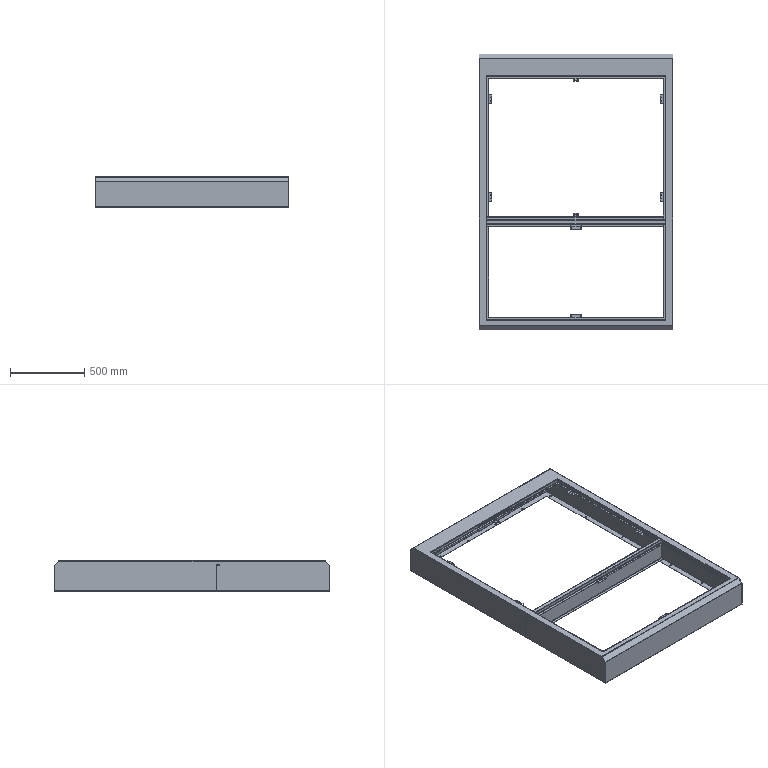Part | NX | features BREP 10 | 10 solids | 442 faces | box 1300 x 1853 x 203 mm | volume 3816472 mm3 | plane 262 | cylinder 164 | spline 16 | commonest cylinder face diameters 6 x58 7 x47 4 x26 5 x16 5.5 x16 8 x1